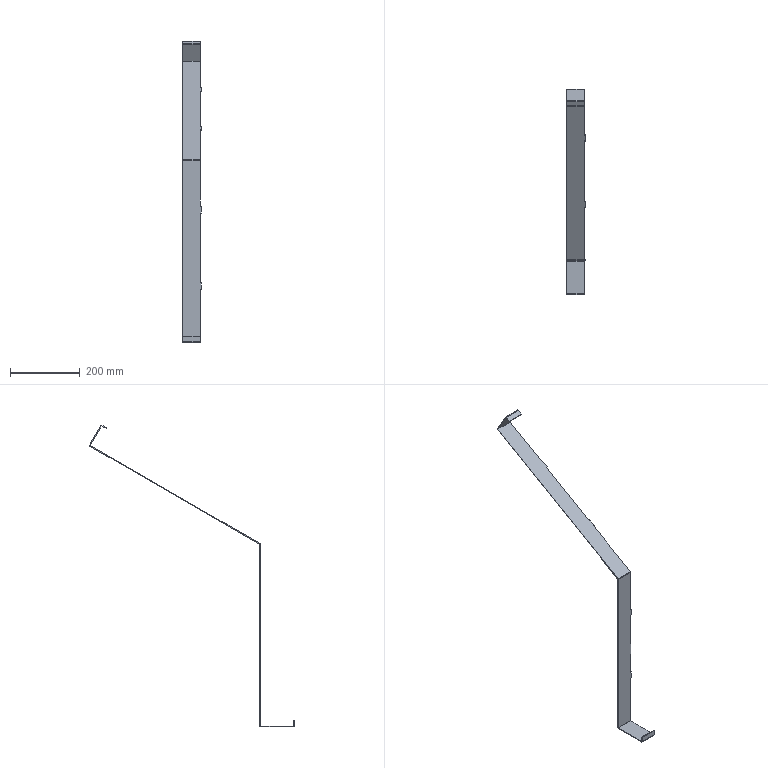Part | STEP file | zzh001 | 1 solid | 44 faces | box 53 x 587.725 x 864.748 mm | volume 128593 mm3 | plane 32 | cylinder 12 | commonest cylinder face diameters 1 x6 5 x6
STEP:
#1=CARTESIAN_POINT('',(50.,493.625,574.029));
#2=VERTEX_POINT('',#1);
#3=CARTESIAN_POINT('',(50.,494.058,573.779));
#4=VERTEX_POINT('',#3);
#5=CARTESIAN_POINT('',(50.,493.625,573.529));
#6=DIRECTION('',(-1.,0.,0.));
#7=DIRECTION('',(0.,0.,1.));
#8=AXIS2_PLACEMENT_3D('',#5,#6,#7);
#9=CIRCLE('',#8,0.5);
#10=EDGE_CURVE('',#2,#4,#9,.T.);
#11=ORIENTED_EDGE('',*,*,#10,.F.);
#12=CARTESIAN_POINT('',(0.,493.625,574.029));
#13=VERTEX_POINT('',#12);
#14=CARTESIAN_POINT('',(50.,493.625,574.029));
#15=DIRECTION('',(-1.,0.,0.));
#16=VECTOR('',#15,1000.);
#17=LINE('',#14,#16);
#18=EDGE_CURVE('',#2,#13,#17,.T.);
#19=ORIENTED_EDGE('',*,*,#18,.T.);
#20=CARTESIAN_POINT('',(0.,494.058,573.779));
#21=VERTEX_POINT('',#20);
#22=CARTESIAN_POINT('',(0.,493.625,573.529));
#23=DIRECTION('',(1.,0.,0.));
#24=DIRECTION('',(0.,0.,1.));
#25=AXIS2_PLACEMENT_3D('',#22,#23,#24);
#26=CIRCLE('',#25,0.5);
#27=EDGE_CURVE('',#21,#13,#26,.T.);
#28=ORIENTED_EDGE('',*,*,#27,.F.);
#29=CARTESIAN_POINT('',(50.,494.058,573.779));
#30=DIRECTION('',(-1.,0.,0.));
#31=VECTOR('',#30,1000.);
#32=LINE('',#29,#31);
#33=EDGE_CURVE('',#4,#21,#32,.T.);
#34=ORIENTED_EDGE('',*,*,#33,.F.);
#35=EDGE_LOOP('',(#11,#19,#28,#34));
#36=FACE_OUTER_BOUND('',#35,.T.);
#37=CARTESIAN_POINT('',(50.,493.625,573.529));
#38=DIRECTION('',(-1.,0.,0.));
#39=DIRECTION('',(0.,0.,1.));
#40=AXIS2_PLACEMENT_3D('',#37,#38,#39);
#41=CYLINDRICAL_SURFACE('',#40,0.5);
#42=ADVANCED_FACE('',(#36),#41,.F.);
#43=CARTESIAN_POINT('',(50.,493.625,576.029));
#44=VERTEX_POINT('',#43);
#45=CARTESIAN_POINT('',(50.,492.375,575.695));
#46=VERTEX_POINT('',#45);
#47=CARTESIAN_POINT('',(50.,493.625,573.529));
#48=DIRECTION('',(1.,0.,0.));
#49=DIRECTION('',(0.,0.,1.));
#50=AXIS2_PLACEMENT_3D('',#47,#48,#49);
#51=CIRCLE('',#50,2.5);
#52=EDGE_CURVE('',#44,#46,#51,.T.);
#53=ORIENTED_EDGE('',*,*,#52,.F.);
#54=CARTESIAN_POINT('',(0.,493.625,576.029));
#55=VERTEX_POINT('',#54);
#56=CARTESIAN_POINT('',(50.,493.625,576.029));
#57=DIRECTION('',(-1.,0.,0.));
#58=VECTOR('',#57,1000.);
#59=LINE('',#56,#58);
#60=EDGE_CURVE('',#44,#55,#59,.T.);
#61=ORIENTED_EDGE('',*,*,#60,.T.);
#62=CARTESIAN_POINT('',(0.,492.375,575.695));
#63=VERTEX_POINT('',#62);
#64=CARTESIAN_POINT('',(0.,493.625,573.529));
#65=DIRECTION('',(-1.,0.,0.));
#66=DIRECTION('',(0.,0.,1.));
#67=AXIS2_PLACEMENT_3D('',#64,#65,#66);
#68=CIRCLE('',#67,2.5);
#69=EDGE_CURVE('',#63,#55,#68,.T.);
#70=ORIENTED_EDGE('',*,*,#69,.F.);
#71=CARTESIAN_POINT('',(50.,492.375,575.695));
#72=DIRECTION('',(1.,0.,0.));
#73=VECTOR('',#72,1000.);
#74=LINE('',#71,#73);
#75=EDGE_CURVE('',#63,#46,#74,.T.);
#76=ORIENTED_EDGE('',*,*,#75,.T.);
#77=EDGE_LOOP('',(#53,#61,#70,#76));
#78=FACE_OUTER_BOUND('',#77,.T.);
#79=CARTESIAN_POINT('',(50.,493.625,573.529));
#80=DIRECTION('',(-1.,0.,0.));
#81=DIRECTION('',(0.,0.,1.));
#82=AXIS2_PLACEMENT_3D('',#79,#80,#81);
#83=CYLINDRICAL_SURFACE('',#82,2.5);
#84=ADVANCED_FACE('',(#78),#83,.T.);
#85=CARTESIAN_POINT('',(50.,396.504,442.748));
#86=VERTEX_POINT('',#85);
#87=CARTESIAN_POINT('',(50.,525.975,517.498));
#88=VERTEX_POINT('',#87);
#89=CARTESIAN_POINT('',(50.,37.7,235.592));
#90=DIRECTION('',(0.,0.866,0.5));
#91=VECTOR('',#90,1000.);
#92=LINE('',#89,#91);
#93=EDGE_CURVE('',#86,#88,#92,.T.);
#94=ORIENTED_EDGE('',*,*,#93,.T.);
#95=CARTESIAN_POINT('',(0.,525.975,517.498));
#96=VERTEX_POINT('',#95);
#97=CARTESIAN_POINT('',(50.,525.975,517.498));
#98=DIRECTION('',(-1.,0.,0.));
#99=VECTOR('',#98,1000.);
#100=LINE('',#97,#99);
#101=EDGE_CURVE('',#88,#96,#100,.T.);
#102=ORIENTED_EDGE('',*,*,#101,.T.);
#103=CARTESIAN_POINT('',(0.,38.95,236.314));
#104=VERTEX_POINT('',#103);
#105=CARTESIAN_POINT('',(0.,37.7,235.592));
#106=DIRECTION('',(0.,-0.866,-0.5));
#107=VECTOR('',#106,1000.);
#108=LINE('',#105,#107);
#109=EDGE_CURVE('',#96,#104,#108,.T.);
#110=ORIENTED_EDGE('',*,*,#109,.T.);
#111=CARTESIAN_POINT('',(50.,38.95,236.314));
#112=VERTEX_POINT('',#111);
#113=CARTESIAN_POINT('',(50.,38.95,236.314));
#114=DIRECTION('',(1.,0.,0.));
#115=VECTOR('',#114,1000.);
#116=LINE('',#113,#115);
#117=EDGE_CURVE('',#104,#112,#116,.T.);
#118=ORIENTED_EDGE('',*,*,#117,.T.);
#119=CARTESIAN_POINT('',(50.,188.658,322.748));
#120=VERTEX_POINT('',#119);
#121=CARTESIAN_POINT('',(50.,37.7,235.592));
#122=DIRECTION('',(0.,0.866,0.5));
#123=VECTOR('',#122,1000.);
#124=LINE('',#121,#123);
#125=EDGE_CURVE('',#112,#120,#124,.T.);
#126=ORIENTED_EDGE('',*,*,#125,.T.);
#127=CARTESIAN_POINT('',(53.,188.658,322.748));
#128=VERTEX_POINT('',#127);
#129=CARTESIAN_POINT('',(50.,188.658,322.748));
#130=DIRECTION('',(1.,0.,0.));
#131=VECTOR('',#130,1000.);
#132=LINE('',#129,#131);
#133=EDGE_CURVE('',#120,#128,#132,.T.);
#134=ORIENTED_EDGE('',*,*,#133,.T.);
#135=CARTESIAN_POINT('',(53.,205.978,332.748));
#136=VERTEX_POINT('',#135);
#137=CARTESIAN_POINT('',(53.,37.7,235.592));
#138=DIRECTION('',(0.,0.866,0.5));
#139=VECTOR('',#138,1000.);
#140=LINE('',#137,#139);
#141=EDGE_CURVE('',#128,#136,#140,.T.);
#142=ORIENTED_EDGE('',*,*,#141,.T.);
#143=CARTESIAN_POINT('',(50.,205.978,332.748));
#144=VERTEX_POINT('',#143);
#145=CARTESIAN_POINT('',(50.,205.978,332.748));
#146=DIRECTION('',(-1.,0.,0.));
#147=VECTOR('',#146,1000.);
#148=LINE('',#145,#147);
#149=EDGE_CURVE('',#136,#144,#148,.T.);
#150=ORIENTED_EDGE('',*,*,#149,.T.);
#151=CARTESIAN_POINT('',(50.,379.183,432.748));
#152=VERTEX_POINT('',#151);
#153=CARTESIAN_POINT('',(50.,37.7,235.592));
#154=DIRECTION('',(0.,0.866,0.5));
#155=VECTOR('',#154,1000.);
#156=LINE('',#153,#155);
#157=EDGE_CURVE('',#144,#152,#156,.T.);
#158=ORIENTED_EDGE('',*,*,#157,.T.);
#159=CARTESIAN_POINT('',(53.,379.183,432.748));
#160=VERTEX_POINT('',#159);
#161=CARTESIAN_POINT('',(50.,379.183,432.748));
#162=DIRECTION('',(1.,0.,0.));
#163=VECTOR('',#162,1000.);
#164=LINE('',#161,#163);
#165=EDGE_CURVE('',#152,#160,#164,.T.);
#166=ORIENTED_EDGE('',*,*,#165,.T.);
#167=CARTESIAN_POINT('',(53.,396.504,442.748));
#168=VERTEX_POINT('',#167);
#169=CARTESIAN_POINT('',(53.,37.7,235.592));
#170=DIRECTION('',(0.,0.866,0.5));
#171=VECTOR('',#170,1000.);
#172=LINE('',#169,#171);
#173=EDGE_CURVE('',#160,#168,#172,.T.);
#174=ORIENTED_EDGE('',*,*,#173,.T.);
#175=CARTESIAN_POINT('',(50.,396.504,442.748));
#176=DIRECTION('',(-1.,0.,0.));
#177=VECTOR('',#176,1000.);
#178=LINE('',#175,#177);
#179=EDGE_CURVE('',#168,#86,#178,.T.);
#180=ORIENTED_EDGE('',*,*,#179,.T.);
#181=EDGE_LOOP('',(#94,#102,#110,#118,#126,#134,#142,#150,#158,#166,#174,#180));
#182=FACE_OUTER_BOUND('',#181,.T.);
#183=CARTESIAN_POINT('',(50.,37.7,235.592));
#184=DIRECTION('',(0.,-0.5,0.866));
#185=DIRECTION('',(0.,-0.866,-0.5));
#186=AXIS2_PLACEMENT_3D('',#183,#184,#185);
#187=PLANE('',#186);
#188=ADVANCED_FACE('',(#182),#187,.T.);
#189=ORIENTED_EDGE('',*,*,#101,.F.);
#190=CARTESIAN_POINT('',(50.,526.158,518.181));
#191=VERTEX_POINT('',#190);
#192=CARTESIAN_POINT('',(50.,525.725,517.931));
#193=DIRECTION('',(-1.,0.,0.));
#194=DIRECTION('',(0.,0.,1.));
#195=AXIS2_PLACEMENT_3D('',#192,#193,#194);
#196=CIRCLE('',#195,0.5);
#197=EDGE_CURVE('',#191,#88,#196,.T.);
#198=ORIENTED_EDGE('',*,*,#197,.F.);
#199=CARTESIAN_POINT('',(0.,526.158,518.181));
#200=VERTEX_POINT('',#199);
#201=CARTESIAN_POINT('',(50.,526.158,518.181));
#202=DIRECTION('',(1.,0.,0.));
#203=VECTOR('',#202,1000.);
#204=LINE('',#201,#203);
#205=EDGE_CURVE('',#200,#191,#204,.T.);
#206=ORIENTED_EDGE('',*,*,#205,.F.);
#207=CARTESIAN_POINT('',(0.,525.725,517.931));
#208=DIRECTION('',(1.,0.,0.));
#209=DIRECTION('',(0.,0.,1.));
#210=AXIS2_PLACEMENT_3D('',#207,#208,#209);
#211=CIRCLE('',#210,0.5);
#212=EDGE_CURVE('',#96,#200,#211,.T.);
#213=ORIENTED_EDGE('',*,*,#212,.F.);
#214=EDGE_LOOP('',(#189,#198,#206,#213));
#215=FACE_OUTER_BOUND('',#214,.T.);
#216=CARTESIAN_POINT('',(50.,525.725,517.931));
#217=DIRECTION('',(-1.,0.,0.));
#218=DIRECTION('',(0.,0.,1.));
#219=AXIS2_PLACEMENT_3D('',#216,#217,#218);
#220=CYLINDRICAL_SURFACE('',#219,0.5);
#221=ADVANCED_FACE('',(#215),#220,.F.);
#222=CARTESIAN_POINT('',(50.,397.504,441.016));
#223=VERTEX_POINT('',#222);
#224=CARTESIAN_POINT('',(50.,526.975,515.766));
#225=VERTEX_POINT('',#224);
#226=CARTESIAN_POINT('',(50.,397.504,441.016));
#227=DIRECTION('',(0.,0.866,0.5));
#228=VECTOR('',#227,1000.);
#229=LINE('',#226,#228);
#230=EDGE_CURVE('',#223,#225,#229,.T.);
#231=ORIENTED_EDGE('',*,*,#230,.T.);
#232=CARTESIAN_POINT('',(50.,527.89,519.181));
#233=VERTEX_POINT('',#232);
#234=CARTESIAN_POINT('',(50.,525.725,517.931));
#235=DIRECTION('',(1.,0.,0.));
#236=DIRECTION('',(0.,0.,1.));
#237=AXIS2_PLACEMENT_3D('',#234,#235,#236);
#238=CIRCLE('',#237,2.5);
#239=EDGE_CURVE('',#225,#233,#238,.T.);
#240=ORIENTED_EDGE('',*,*,#239,.T.);
#241=CARTESIAN_POINT('',(50.,495.79,574.779));
#242=VERTEX_POINT('',#241);
#243=CARTESIAN_POINT('',(50.,527.89,519.181));
#244=DIRECTION('',(0.,-0.5,0.866));
#245=VECTOR('',#244,1000.);
#246=LINE('',#243,#245);
#247=EDGE_CURVE('',#233,#242,#246,.T.);
#248=ORIENTED_EDGE('',*,*,#247,.T.);
#249=CARTESIAN_POINT('',(50.,493.625,573.529));
#250=DIRECTION('',(1.,0.,0.));
#251=DIRECTION('',(0.,0.,1.));
#252=AXIS2_PLACEMENT_3D('',#249,#250,#251);
#253=CIRCLE('',#252,2.5);
#254=EDGE_CURVE('',#242,#44,#253,.T.);
#255=ORIENTED_EDGE('',*,*,#254,.T.);
#256=ORIENTED_EDGE('',*,*,#52,.T.);
#257=CARTESIAN_POINT('',(50.,479.817,568.445));
#258=VERTEX_POINT('',#257);
#259=CARTESIAN_POINT('',(50.,492.375,575.695));
#260=DIRECTION('',(0.,-0.866,-0.5));
#261=VECTOR('',#260,1000.);
#262=LINE('',#259,#261);
#263=EDGE_CURVE('',#46,#258,#262,.T.);
#264=ORIENTED_EDGE('',*,*,#263,.T.);
#265=CARTESIAN_POINT('',(50.,480.817,566.713));
#266=VERTEX_POINT('',#265);
#267=CARTESIAN_POINT('',(50.,479.817,568.445));
#268=DIRECTION('',(0.,0.5,-0.866));
#269=VECTOR('',#268,1000.);
#270=LINE('',#267,#269);
#271=EDGE_CURVE('',#258,#266,#270,.T.);
#272=ORIENTED_EDGE('',*,*,#271,.T.);
#273=CARTESIAN_POINT('',(50.,493.375,573.963));
#274=VERTEX_POINT('',#273);
#275=CARTESIAN_POINT('',(50.,493.808,574.213));
#276=DIRECTION('',(0.,-0.866,-0.5));
#277=VECTOR('',#276,1000.);
#278=LINE('',#275,#277);
#279=EDGE_CURVE('',#274,#266,#278,.T.);
#280=ORIENTED_EDGE('',*,*,#279,.F.);
#281=CARTESIAN_POINT('',(50.,493.625,573.529));
#282=DIRECTION('',(-1.,0.,0.));
#283=DIRECTION('',(0.,0.,1.));
#284=AXIS2_PLACEMENT_3D('',#281,#282,#283);
#285=CIRCLE('',#284,0.5);
#286=EDGE_CURVE('',#274,#2,#285,.T.);
#287=ORIENTED_EDGE('',*,*,#286,.T.);
#288=ORIENTED_EDGE('',*,*,#10,.T.);
#289=CARTESIAN_POINT('',(50.,526.408,517.748));
#290=DIRECTION('',(0.,-0.5,0.866));
#291=VECTOR('',#290,1000.);
#292=LINE('',#289,#291);
#293=EDGE_CURVE('',#191,#4,#292,.T.);
#294=ORIENTED_EDGE('',*,*,#293,.F.);
#295=ORIENTED_EDGE('',*,*,#197,.T.);
#296=ORIENTED_EDGE('',*,*,#93,.F.);
#297=CARTESIAN_POINT('',(50.,396.504,442.748));
#298=DIRECTION('',(0.,0.5,-0.866));
#299=VECTOR('',#298,1000.);
#300=LINE('',#297,#299);
#301=EDGE_CURVE('',#86,#223,#300,.T.);
#302=ORIENTED_EDGE('',*,*,#301,.T.);
#303=EDGE_LOOP('',(#231,#240,#248,#255,#256,#264,#272,#280,#287,#288,#294,#295,#296,#302));
#304=FACE_OUTER_BOUND('',#303,.T.);
#305=CARTESIAN_POINT('',(50.,39.7,234.149));
#306=DIRECTION('',(1.,0.,0.));
#307=DIRECTION('',(0.,0.,-1.));
#308=AXIS2_PLACEMENT_3D('',#305,#306,#307);
#309=PLANE('',#308);
#310=ADVANCED_FACE('',(#304),#309,.T.);
#311=ORIENTED_EDGE('',*,*,#179,.F.);
#312=CARTESIAN_POINT('',(53.,397.504,441.016));
#313=VERTEX_POINT('',#312);
#314=CARTESIAN_POINT('',(53.,396.504,442.748));
#315=DIRECTION('',(0.,-0.5,0.866));
#316=VECTOR('',#315,1000.);
#317=LINE('',#314,#316);
#318=EDGE_CURVE('',#313,#168,#317,.T.);
#319=ORIENTED_EDGE('',*,*,#318,.F.);
#320=CARTESIAN_POINT('',(53.,397.504,441.016));
#321=DIRECTION('',(1.,0.,0.));
#322=VECTOR('',#321,1000.);
#323=LINE('',#320,#322);
#324=EDGE_CURVE('',#223,#313,#323,.T.);
#325=ORIENTED_EDGE('',*,*,#324,.F.);
#326=ORIENTED_EDGE('',*,*,#301,.F.);
#327=EDGE_LOOP('',(#311,#319,#325,#326));
#328=FACE_OUTER_BOUND('',#327,.T.);
#329=CARTESIAN_POINT('',(53.,396.504,442.748));
#330=DIRECTION('',(0.,-0.866,-0.5));
#331=DIRECTION('',(0.,0.5,-0.866));
#332=AXIS2_PLACEMENT_3D('',#329,#330,#331);
#333=PLANE('',#332);
#334=ADVANCED_FACE('',(#328),#333,.F.);
#335=ORIENTED_EDGE('',*,*,#173,.F.);
#336=CARTESIAN_POINT('',(53.,380.183,431.016));
#337=VERTEX_POINT('',#336);
#338=CARTESIAN_POINT('',(53.,380.183,431.016));
#339=DIRECTION('',(0.,-0.5,0.866));
#340=VECTOR('',#339,1000.);
#341=LINE('',#338,#340);
#342=EDGE_CURVE('',#337,#160,#341,.T.);
#343=ORIENTED_EDGE('',*,*,#342,.F.);
#344=CARTESIAN_POINT('',(53.,397.504,441.016));
#345=DIRECTION('',(0.,-0.866,-0.5));
#346=VECTOR('',#345,1000.);
#347=LINE('',#344,#346);
#348=EDGE_CURVE('',#313,#337,#347,.T.);
#349=ORIENTED_EDGE('',*,*,#348,.F.);
#350=ORIENTED_EDGE('',*,*,#318,.T.);
#351=EDGE_LOOP('',(#335,#343,#349,#350));
#352=FACE_OUTER_BOUND('',#351,.T.);
#353=CARTESIAN_POINT('',(53.,0.,0.));
#354=DIRECTION('',(-1.,0.,0.));
#355=DIRECTION('',(0.,0.,1.));
#356=AXIS2_PLACEMENT_3D('',#353,#354,#355);
#357=PLANE('',#356);
#358=ADVANCED_FACE('',(#352),#357,.F.);
#359=CARTESIAN_POINT('',(50.,380.183,431.016));
#360=VERTEX_POINT('',#359);
#361=CARTESIAN_POINT('',(53.,380.183,431.016));
#362=DIRECTION('',(-1.,0.,0.));
#363=VECTOR('',#362,1000.);
#364=LINE('',#361,#363);
#365=EDGE_CURVE('',#337,#360,#364,.T.);
#366=ORIENTED_EDGE('',*,*,#365,.F.);
#367=ORIENTED_EDGE('',*,*,#342,.T.);
#368=ORIENTED_EDGE('',*,*,#165,.F.);
#369=CARTESIAN_POINT('',(50.,379.183,432.748));
#370=DIRECTION('',(0.,-0.5,0.866));
#371=VECTOR('',#370,1000.);
#372=LINE('',#369,#371);
#373=EDGE_CURVE('',#360,#152,#372,.T.);
#374=ORIENTED_EDGE('',*,*,#373,.F.);
#375=EDGE_LOOP('',(#366,#367,#368,#374));
#376=FACE_OUTER_BOUND('',#375,.T.);
#377=CARTESIAN_POINT('',(53.,379.183,432.748));
#378=DIRECTION('',(0.,0.866,0.5));
#379=DIRECTION('',(0.,-0.5,0.866));
#380=AXIS2_PLACEMENT_3D('',#377,#378,#379);
#381=PLANE('',#380);
#382=ADVANCED_FACE('',(#376),#381,.F.);
#383=CARTESIAN_POINT('',(50.,206.978,331.016));
#384=VERTEX_POINT('',#383);
#385=CARTESIAN_POINT('',(50.,206.978,331.016));
#386=DIRECTION('',(0.,0.866,0.5));
#387=VECTOR('',#386,1000.);
#388=LINE('',#385,#387);
#389=EDGE_CURVE('',#384,#360,#388,.T.);
#390=ORIENTED_EDGE('',*,*,#389,.T.);
#391=ORIENTED_EDGE('',*,*,#373,.T.);
#392=ORIENTED_EDGE('',*,*,#157,.F.);
#393=CARTESIAN_POINT('',(50.,205.978,332.748));
#394=DIRECTION('',(0.,0.5,-0.866));
#395=VECTOR('',#394,1000.);
#396=LINE('',#393,#395);
#397=EDGE_CURVE('',#144,#384,#396,.T.);
#398=ORIENTED_EDGE('',*,*,#397,.T.);
#399=EDGE_LOOP('',(#390,#391,#392,#398));
#400=FACE_OUTER_BOUND('',#399,.T.);
#401=CARTESIAN_POINT('',(50.,39.7,234.149));
#402=DIRECTION('',(1.,0.,0.));
#403=DIRECTION('',(0.,0.,-1.));
#404=AXIS2_PLACEMENT_3D('',#401,#402,#403);
#405=PLANE('',#404);
#406=ADVANCED_FACE('',(#400),#405,.T.);
#407=ORIENTED_EDGE('',*,*,#149,.F.);
#408=CARTESIAN_POINT('',(53.,206.978,331.016));
#409=VERTEX_POINT('',#408);
#410=CARTESIAN_POINT('',(53.,205.978,332.748));
#411=DIRECTION('',(0.,-0.5,0.866));
#412=VECTOR('',#411,1000.);
#413=LINE('',#410,#412);
#414=EDGE_CURVE('',#409,#136,#413,.T.);
#415=ORIENTED_EDGE('',*,*,#414,.F.);
#416=CARTESIAN_POINT('',(53.,206.978,331.016));
#417=DIRECTION('',(1.,0.,0.));
#418=VECTOR('',#417,1000.);
#419=LINE('',#416,#418);
#420=EDGE_CURVE('',#384,#409,#419,.T.);
#421=ORIENTED_EDGE('',*,*,#420,.F.);
#422=ORIENTED_EDGE('',*,*,#397,.F.);
#423=EDGE_LOOP('',(#407,#415,#421,#422));
#424=FACE_OUTER_BOUND('',#423,.T.);
#425=CARTESIAN_POINT('',(53.,205.978,332.748));
#426=DIRECTION('',(0.,-0.866,-0.5));
#427=DIRECTION('',(0.,0.5,-0.866));
#428=AXIS2_PLACEMENT_3D('',#425,#426,#427);
#429=PLANE('',#428);
#430=ADVANCED_FACE('',(#424),#429,.F.);
#431=ORIENTED_EDGE('',*,*,#141,.F.);
#432=CARTESIAN_POINT('',(53.,189.658,321.016));
#433=VERTEX_POINT('',#432);
#434=CARTESIAN_POINT('',(53.,189.658,321.016));
#435=DIRECTION('',(0.,-0.5,0.866));
#436=VECTOR('',#435,1000.);
#437=LINE('',#434,#436);
#438=EDGE_CURVE('',#433,#128,#437,.T.);
#439=ORIENTED_EDGE('',*,*,#438,.F.);
#440=CARTESIAN_POINT('',(53.,206.978,331.016));
#441=DIRECTION('',(0.,-0.866,-0.5));
#442=VECTOR('',#441,1000.);
#443=LINE('',#440,#442);
#444=EDGE_CURVE('',#409,#433,#443,.T.);
#445=ORIENTED_EDGE('',*,*,#444,.F.);
#446=ORIENTED_EDGE('',*,*,#414,.T.);
#447=EDGE_LOOP('',(#431,#439,#445,#446));
#448=FACE_OUTER_BOUND('',#447,.T.);
#449=CARTESIAN_POINT('',(53.,0.,0.));
#450=DIRECTION('',(-1.,0.,0.));
#451=DIRECTION('',(0.,0.,1.));
#452=AXIS2_PLACEMENT_3D('',#449,#450,#451);
#453=PLANE('',#452);
#454=ADVANCED_FACE('',(#448),#453,.F.);
#455=CARTESIAN_POINT('',(50.,189.658,321.016));
#456=VERTEX_POINT('',#455);
#457=CARTESIAN_POINT('',(53.,189.658,321.016));
#458=DIRECTION('',(-1.,0.,0.));
#459=VECTOR('',#458,1000.);
#460=LINE('',#457,#459);
#461=EDGE_CURVE('',#433,#456,#460,.T.);
#462=ORIENTED_EDGE('',*,*,#461,.F.);
#463=ORIENTED_EDGE('',*,*,#438,.T.);
#464=ORIENTED_EDGE('',*,*,#133,.F.);
#465=CARTESIAN_POINT('',(50.,188.658,322.748));
#466=DIRECTION('',(0.,-0.5,0.866));
#467=VECTOR('',#466,1000.);
#468=LINE('',#465,#467);
#469=EDGE_CURVE('',#456,#120,#468,.T.);
#470=ORIENTED_EDGE('',*,*,#469,.F.);
#471=EDGE_LOOP('',(#462,#463,#464,#470));
#472=FACE_OUTER_BOUND('',#471,.T.);
#473=CARTESIAN_POINT('',(53.,188.658,322.748));
#474=DIRECTION('',(0.,0.866,0.5));
#475=DIRECTION('',(0.,-0.5,0.866));
#476=AXIS2_PLACEMENT_3D('',#473,#474,#475);
#477=PLANE('',#476);
#478=ADVANCED_FACE('',(#472),#477,.F.);
#479=ORIENTED_EDGE('',*,*,#125,.F.);
#480=CARTESIAN_POINT('',(50.,37.7,234.149));
#481=VERTEX_POINT('',#480);
#482=CARTESIAN_POINT('',(50.,40.2,234.149));
#483=DIRECTION('',(-1.,0.,0.));
#484=DIRECTION('',(0.,0.,1.));
#485=AXIS2_PLACEMENT_3D('',#482,#483,#484);
#486=CIRCLE('',#485,2.5);
#487=EDGE_CURVE('',#481,#112,#486,.T.);
#488=ORIENTED_EDGE('',*,*,#487,.F.);
#489=CARTESIAN_POINT('',(50.,37.7,103.281));
#490=VERTEX_POINT('',#489);
#491=CARTESIAN_POINT('',(50.,37.7,-286.719));
#492=DIRECTION('',(0.,0.,1.));
#493=VECTOR('',#492,1000.);
#494=LINE('',#491,#493);
#495=EDGE_CURVE('',#490,#481,#494,.T.);
#496=ORIENTED_EDGE('',*,*,#495,.F.);
#497=CARTESIAN_POINT('',(50.,39.7,103.281));
#498=VERTEX_POINT('',#497);
#499=CARTESIAN_POINT('',(50.,37.2,103.281));
#500=DIRECTION('',(0.,1.,0.));
#501=VECTOR('',#500,1000.);
#502=LINE('',#499,#501);
#503=EDGE_CURVE('',#490,#498,#502,.T.);
#504=ORIENTED_EDGE('',*,*,#503,.T.);
#505=CARTESIAN_POINT('',(50.,39.7,234.149));
#506=VERTEX_POINT('',#505);
#507=CARTESIAN_POINT('',(50.,39.7,-288.719));
#508=DIRECTION('',(0.,0.,1.));
#509=VECTOR('',#508,1000.);
#510=LINE('',#507,#509);
#511=EDGE_CURVE('',#498,#506,#510,.T.);
#512=ORIENTED_EDGE('',*,*,#511,.T.);
#513=CARTESIAN_POINT('',(50.,39.95,234.582));
#514=VERTEX_POINT('',#513);
#515=CARTESIAN_POINT('',(50.,40.2,234.149));
#516=DIRECTION('',(-1.,0.,0.));
#517=DIRECTION('',(0.,0.,1.));
#518=AXIS2_PLACEMENT_3D('',#515,#516,#517);
#519=CIRCLE('',#518,0.5);
#520=EDGE_CURVE('',#506,#514,#519,.T.);
#521=ORIENTED_EDGE('',*,*,#520,.T.);
#522=CARTESIAN_POINT('',(50.,39.95,234.582));
#523=DIRECTION('',(0.,0.866,0.5));
#524=VECTOR('',#523,1000.);
#525=LINE('',#522,#524);
#526=EDGE_CURVE('',#514,#456,#525,.T.);
#527=ORIENTED_EDGE('',*,*,#526,.T.);
#528=ORIENTED_EDGE('',*,*,#469,.T.);
#529=EDGE_LOOP('',(#479,#488,#496,#504,#512,#521,#527,#528));
#530=FACE_OUTER_BOUND('',#529,.T.);
#531=CARTESIAN_POINT('',(50.,39.7,234.149));
#532=DIRECTION('',(1.,0.,0.));
#533=DIRECTION('',(0.,0.,-1.));
#534=AXIS2_PLACEMENT_3D('',#531,#532,#533);
#535=PLANE('',#534);
#536=ADVANCED_FACE('',(#530),#535,.T.);
#537=ORIENTED_EDGE('',*,*,#487,.T.);
#538=ORIENTED_EDGE('',*,*,#117,.F.);
#539=CARTESIAN_POINT('',(0.,37.7,234.149));
#540=VERTEX_POINT('',#539);
#541=CARTESIAN_POINT('',(0.,40.2,234.149));
#542=DIRECTION('',(1.,0.,0.));
#543=DIRECTION('',(0.,0.,1.));
#544=AXIS2_PLACEMENT_3D('',#541,#542,#543);
#545=CIRCLE('',#544,2.5);
#546=EDGE_CURVE('',#104,#540,#545,.T.);
#547=ORIENTED_EDGE('',*,*,#546,.T.);
#548=CARTESIAN_POINT('',(50.,37.7,234.149));
#549=DIRECTION('',(1.,0.,0.));
#550=VECTOR('',#549,1000.);
#551=LINE('',#548,#550);
#552=EDGE_CURVE('',#540,#481,#551,.T.);
#553=ORIENTED_EDGE('',*,*,#552,.T.);
#554=EDGE_LOOP('',(#537,#538,#547,#553));
#555=FACE_OUTER_BOUND('',#554,.T.);
#556=CARTESIAN_POINT('',(50.,40.2,234.149));
#557=DIRECTION('',(-1.,0.,0.));
#558=DIRECTION('',(0.,0.,1.));
#559=AXIS2_PLACEMENT_3D('',#556,#557,#558);
#560=CYLINDRICAL_SURFACE('',#559,2.5);
#561=ADVANCED_FACE('',(#555),#560,.T.);
#562=CARTESIAN_POINT('',(0.,526.975,515.766));
#563=VERTEX_POINT('',#562);
#564=CARTESIAN_POINT('',(0.,39.95,234.582));
#565=VERTEX_POINT('',#564);
#566=CARTESIAN_POINT('',(0.,526.975,515.766));
#567=DIRECTION('',(0.,-0.866,-0.5));
#568=VECTOR('',#567,1000.);
#569=LINE('',#566,#568);
#570=EDGE_CURVE('',#563,#565,#569,.T.);
#571=ORIENTED_EDGE('',*,*,#570,.T.);
#572=CARTESIAN_POINT('',(0.,39.7,234.149));
#573=VERTEX_POINT('',#572);
#574=CARTESIAN_POINT('',(0.,40.2,234.149));
#575=DIRECTION('',(1.,0.,0.));
#576=DIRECTION('',(0.,0.,1.));
#577=AXIS2_PLACEMENT_3D('',#574,#575,#576);
#578=CIRCLE('',#577,0.5);
#579=EDGE_CURVE('',#565,#573,#578,.T.);
#580=ORIENTED_EDGE('',*,*,#579,.T.);
#581=CARTESIAN_POINT('',(0.,39.7,-286.219));
#582=VERTEX_POINT('',#581);
#583=CARTESIAN_POINT('',(0.,39.7,234.582));
#584=DIRECTION('',(0.,0.,-1.));
#585=VECTOR('',#584,1000.);
#586=LINE('',#583,#585);
#587=EDGE_CURVE('',#573,#582,#586,.T.);
#588=ORIENTED_EDGE('',*,*,#587,.T.);
#589=CARTESIAN_POINT('',(0.,37.2,-288.719));
#590=VERTEX_POINT('',#589);
#591=CARTESIAN_POINT('',(0.,37.2,-286.219));
#592=DIRECTION('',(-1.,0.,0.));
#593=DIRECTION('',(0.,0.,1.));
#594=AXIS2_PLACEMENT_3D('',#591,#592,#593);
#595=CIRCLE('',#594,2.5);
#596=EDGE_CURVE('',#582,#590,#595,.T.);
#597=ORIENTED_EDGE('',*,*,#596,.T.);
#598=CARTESIAN_POINT('',(0.,-57.,-288.719));
#599=VERTEX_POINT('',#598);
#600=CARTESIAN_POINT('',(0.,39.7,-288.719));
#601=DIRECTION('',(0.,-1.,0.));
#602=VECTOR('',#601,1000.);
#603=LINE('',#600,#602);
#604=EDGE_CURVE('',#590,#599,#603,.T.);
#605=ORIENTED_EDGE('',*,*,#604,.T.);
#606=CARTESIAN_POINT('',(0.,-59.5,-286.219));
#607=VERTEX_POINT('',#606);
#608=CARTESIAN_POINT('',(0.,-57.,-286.219));
#609=DIRECTION('',(-1.,0.,0.));
#610=DIRECTION('',(0.,0.,1.));
#611=AXIS2_PLACEMENT_3D('',#608,#609,#610);
#612=CIRCLE('',#611,2.5);
#613=EDGE_CURVE('',#599,#607,#612,.T.);
#614=ORIENTED_EDGE('',*,*,#613,.T.);
#615=CARTESIAN_POINT('',(0.,-59.5,-271.719));
#616=VERTEX_POINT('',#615);
#617=CARTESIAN_POINT('',(0.,-59.5,-288.719));
#618=DIRECTION('',(0.,0.,1.));
#619=VECTOR('',#618,1000.);
#620=LINE('',#617,#619);
#621=EDGE_CURVE('',#607,#616,#620,.T.);
#622=ORIENTED_EDGE('',*,*,#621,.T.);
#623=CARTESIAN_POINT('',(0.,-57.5,-271.719));
#624=VERTEX_POINT('',#623);
#625=CARTESIAN_POINT('',(0.,-59.5,-271.719));
#626=DIRECTION('',(0.,-1.,0.));
#627=VECTOR('',#626,1000.);
#628=LINE('',#625,#627);
#629=EDGE_CURVE('',#624,#616,#628,.T.);
#630=ORIENTED_EDGE('',*,*,#629,.F.);
#631=CARTESIAN_POINT('',(0.,-57.5,-286.219));
#632=VERTEX_POINT('',#631);
#633=CARTESIAN_POINT('',(0.,-57.5,-286.719));
#634=DIRECTION('',(0.,0.,1.));
#635=VECTOR('',#634,1000.);
#636=LINE('',#633,#635);
#637=EDGE_CURVE('',#632,#624,#636,.T.);
#638=ORIENTED_EDGE('',*,*,#637,.F.);
#639=CARTESIAN_POINT('',(0.,-57.,-286.719));
#640=VERTEX_POINT('',#639);
#641=CARTESIAN_POINT('',(0.,-57.,-286.219));
#642=DIRECTION('',(1.,0.,0.));
#643=DIRECTION('',(0.,0.,1.));
#644=AXIS2_PLACEMENT_3D('',#641,#642,#643);
#645=CIRCLE('',#644,0.5);
#646=EDGE_CURVE('',#632,#640,#645,.T.);
#647=ORIENTED_EDGE('',*,*,#646,.T.);
#648=CARTESIAN_POINT('',(0.,37.2,-286.719));
#649=VERTEX_POINT('',#648);
#650=CARTESIAN_POINT('',(0.,-52.5,-286.719));
#651=DIRECTION('',(0.,-1.,0.));
#652=VECTOR('',#651,1000.);
#653=LINE('',#650,#652);
#654=EDGE_CURVE('',#649,#640,#653,.T.);
#655=ORIENTED_EDGE('',*,*,#654,.F.);
#656=CARTESIAN_POINT('',(0.,37.7,-286.219));
#657=VERTEX_POINT('',#656);
#658=CARTESIAN_POINT('',(0.,37.2,-286.219));
#659=DIRECTION('',(1.,0.,0.));
#660=DIRECTION('',(0.,0.,1.));
#661=AXIS2_PLACEMENT_3D('',#658,#659,#660);
#662=CIRCLE('',#661,0.5);
#663=EDGE_CURVE('',#649,#657,#662,.T.);
#664=ORIENTED_EDGE('',*,*,#663,.T.);
#665=CARTESIAN_POINT('',(0.,37.7,-286.719));
#666=DIRECTION('',(0.,0.,-1.));
#667=VECTOR('',#666,1000.);
#668=LINE('',#665,#667);
#669=EDGE_CURVE('',#540,#657,#668,.T.);
#670=ORIENTED_EDGE('',*,*,#669,.F.);
#671=ORIENTED_EDGE('',*,*,#546,.F.);
#672=ORIENTED_EDGE('',*,*,#109,.F.);
#673=ORIENTED_EDGE('',*,*,#212,.T.);
#674=CARTESIAN_POINT('',(0.,526.408,517.748));
#675=DIRECTION('',(0.,0.5,-0.866));
#676=VECTOR('',#675,1000.);
#677=LINE('',#674,#676);
#678=EDGE_CURVE('',#21,#200,#677,.T.);
#679=ORIENTED_EDGE('',*,*,#678,.F.);
#680=ORIENTED_EDGE('',*,*,#27,.T.);
#681=CARTESIAN_POINT('',(0.,493.375,573.963));
#682=VERTEX_POINT('',#681);
#683=CARTESIAN_POINT('',(0.,493.625,573.529));
#684=DIRECTION('',(1.,0.,0.));
#685=DIRECTION('',(0.,0.,1.));
#686=AXIS2_PLACEMENT_3D('',#683,#684,#685);
#687=CIRCLE('',#686,0.5);
#688=EDGE_CURVE('',#13,#682,#687,.T.);
#689=ORIENTED_EDGE('',*,*,#688,.T.);
#690=CARTESIAN_POINT('',(0.,480.817,566.713));
#691=VERTEX_POINT('',#690);
#692=CARTESIAN_POINT('',(0.,493.808,574.213));
#693=DIRECTION('',(0.,0.866,0.5));
#694=VECTOR('',#693,1000.);
#695=LINE('',#692,#694);
#696=EDGE_CURVE('',#691,#682,#695,.T.);
#697=ORIENTED_EDGE('',*,*,#696,.F.);
#698=CARTESIAN_POINT('',(0.,479.817,568.445));
#699=VERTEX_POINT('',#698);
#700=CARTESIAN_POINT('',(0.,480.817,566.713));
#701=DIRECTION('',(0.,-0.5,0.866));
#702=VECTOR('',#701,1000.);
#703=LINE('',#700,#702);
#704=EDGE_CURVE('',#691,#699,#703,.T.);
#705=ORIENTED_EDGE('',*,*,#704,.T.);
#706=CARTESIAN_POINT('',(0.,479.817,568.445));
#707=DIRECTION('',(0.,0.866,0.5));
#708=VECTOR('',#707,1000.);
#709=LINE('',#706,#708);
#710=EDGE_CURVE('',#699,#63,#709,.T.);
#711=ORIENTED_EDGE('',*,*,#710,.T.);
#712=ORIENTED_EDGE('',*,*,#69,.T.);
#713=CARTESIAN_POINT('',(0.,495.79,574.779));
#714=VERTEX_POINT('',#713);
#715=CARTESIAN_POINT('',(0.,493.625,573.529));
#716=DIRECTION('',(-1.,0.,0.));
#717=DIRECTION('',(0.,0.,1.));
#718=AXIS2_PLACEMENT_3D('',#715,#716,#717);
#719=CIRCLE('',#718,2.5);
#720=EDGE_CURVE('',#55,#714,#719,.T.);
#721=ORIENTED_EDGE('',*,*,#720,.T.);
#722=CARTESIAN_POINT('',(0.,527.89,519.181));
#723=VERTEX_POINT('',#722);
#724=CARTESIAN_POINT('',(0.,495.79,574.779));
#725=DIRECTION('',(0.,0.5,-0.866));
#726=VECTOR('',#725,1000.);
#727=LINE('',#724,#726);
#728=EDGE_CURVE('',#714,#723,#727,.T.);
#729=ORIENTED_EDGE('',*,*,#728,.T.);
#730=CARTESIAN_POINT('',(0.,525.725,517.931));
#731=DIRECTION('',(-1.,0.,0.));
#732=DIRECTION('',(0.,0.,1.));
#733=AXIS2_PLACEMENT_3D('',#730,#731,#732);
#734=CIRCLE('',#733,2.5);
#735=EDGE_CURVE('',#723,#563,#734,.T.);
#736=ORIENTED_EDGE('',*,*,#735,.T.);
#737=EDGE_LOOP('',(#571,#580,#588,#597,#605,#614,#622,#630,#638,#647,#655,#664,#670,#671,#672,#673,#679,#680,#689,#697,#705,#711,#712,#721,#729,#736));
#738=FACE_OUTER_BOUND('',#737,.T.);
#739=CARTESIAN_POINT('',(0.,527.89,519.181));
#740=DIRECTION('',(-1.,0.,0.));
#741=DIRECTION('',(0.,0.,1.));
#742=AXIS2_PLACEMENT_3D('',#739,#740,#741);
#743=PLANE('',#742);
#744=ADVANCED_FACE('',(#738),#743,.T.);
#745=ORIENTED_EDGE('',*,*,#293,.T.);
#746=ORIENTED_EDGE('',*,*,#33,.T.);
#747=ORIENTED_EDGE('',*,*,#678,.T.);
#748=ORIENTED_EDGE('',*,*,#205,.T.);
#749=EDGE_LOOP('',(#745,#746,#747,#748));
#750=FACE_OUTER_BOUND('',#749,.T.);
#751=CARTESIAN_POINT('',(50.,526.408,517.748));
#752=DIRECTION('',(0.,-0.866,-0.5));
#753=DIRECTION('',(0.,0.5,-0.866));
#754=AXIS2_PLACEMENT_3D('',#751,#752,#753);
#755=PLANE('',#754);
#756=ADVANCED_FACE('',(#750),#755,.T.);
#757=CARTESIAN_POINT('',(50.,526.975,515.766));
#758=DIRECTION('',(-1.,0.,0.));
#759=VECTOR('',#758,1000.);
#760=LINE('',#757,#759);
#761=EDGE_CURVE('',#225,#563,#760,.T.);
#762=ORIENTED_EDGE('',*,*,#761,.F.);
#763=ORIENTED_EDGE('',*,*,#230,.F.);
#764=ORIENTED_EDGE('',*,*,#324,.T.);
#765=ORIENTED_EDGE('',*,*,#348,.T.);
#766=ORIENTED_EDGE('',*,*,#365,.T.);
#767=ORIENTED_EDGE('',*,*,#389,.F.);
#768=ORIENTED_EDGE('',*,*,#420,.T.);
#769=ORIENTED_EDGE('',*,*,#444,.T.);
#770=ORIENTED_EDGE('',*,*,#461,.T.);
#771=ORIENTED_EDGE('',*,*,#526,.F.);
#772=CARTESIAN_POINT('',(50.,39.95,234.582));
#773=DIRECTION('',(1.,0.,0.));
#774=VECTOR('',#773,1000.);
#775=LINE('',#772,#774);
#776=EDGE_CURVE('',#565,#514,#775,.T.);
#777=ORIENTED_EDGE('',*,*,#776,.F.);
#778=ORIENTED_EDGE('',*,*,#570,.F.);
#779=EDGE_LOOP('',(#762,#763,#764,#765,#766,#767,#768,#769,#770,#771,#777,#778));
#780=FACE_OUTER_BOUND('',#779,.T.);
#781=CARTESIAN_POINT('',(50.,38.7,233.86));
#782=DIRECTION('',(0.,-0.5,0.866));
#783=DIRECTION('',(0.,-0.866,-0.5));
#784=AXIS2_PLACEMENT_3D('',#781,#782,#783);
#785=PLANE('',#784);
#786=ADVANCED_FACE('',(#780),#785,.F.);
#787=ORIENTED_EDGE('',*,*,#495,.T.);
#788=ORIENTED_EDGE('',*,*,#552,.F.);
#789=ORIENTED_EDGE('',*,*,#669,.T.);
#790=CARTESIAN_POINT('',(50.,37.7,-286.219));
#791=VERTEX_POINT('',#790);
#792=CARTESIAN_POINT('',(50.,37.7,-286.219));
#793=DIRECTION('',(1.,0.,0.));
#794=VECTOR('',#793,1000.);
#795=LINE('',#792,#794);
#796=EDGE_CURVE('',#657,#791,#795,.T.);
#797=ORIENTED_EDGE('',*,*,#796,.T.);
#798=CARTESIAN_POINT('',(50.,37.7,-136.719));
#799=VERTEX_POINT('',#798);
#800=CARTESIAN_POINT('',(50.,37.7,-286.719));
#801=DIRECTION('',(0.,0.,1.));
#802=VECTOR('',#801,1000.);
#803=LINE('',#800,#802);
#804=EDGE_CURVE('',#791,#799,#803,.T.);
#805=ORIENTED_EDGE('',*,*,#804,.T.);
#806=CARTESIAN_POINT('',(53.,37.7,-136.719));
#807=VERTEX_POINT('',#806);
#808=CARTESIAN_POINT('',(50.,37.7,-136.719));
#809=DIRECTION('',(1.,0.,0.));
#810=VECTOR('',#809,1000.);
#811=LINE('',#808,#810);
#812=EDGE_CURVE('',#799,#807,#811,.T.);
#813=ORIENTED_EDGE('',*,*,#812,.T.);
#814=CARTESIAN_POINT('',(53.,37.7,-116.719));
#815=VERTEX_POINT('',#814);
#816=CARTESIAN_POINT('',(53.,37.7,-286.719));
#817=DIRECTION('',(0.,0.,1.));
#818=VECTOR('',#817,1000.);
#819=LINE('',#816,#818);
#820=EDGE_CURVE('',#807,#815,#819,.T.);
#821=ORIENTED_EDGE('',*,*,#820,.T.);
#822=CARTESIAN_POINT('',(50.,37.7,-116.719));
#823=VERTEX_POINT('',#822);
#824=CARTESIAN_POINT('',(50.,37.7,-116.719));
#825=DIRECTION('',(-1.,0.,0.));
#826=VECTOR('',#825,1000.);
#827=LINE('',#824,#826);
#828=EDGE_CURVE('',#815,#823,#827,.T.);
#829=ORIENTED_EDGE('',*,*,#828,.T.);
#830=CARTESIAN_POINT('',(50.,37.7,83.281));
#831=VERTEX_POINT('',#830);
#832=CARTESIAN_POINT('',(50.,37.7,-286.719));
#833=DIRECTION('',(0.,0.,1.));
#834=VECTOR('',#833,1000.);
#835=LINE('',#832,#834);
#836=EDGE_CURVE('',#823,#831,#835,.T.);
#837=ORIENTED_EDGE('',*,*,#836,.T.);
#838=CARTESIAN_POINT('',(53.,37.7,83.281));
#839=VERTEX_POINT('',#838);
#840=CARTESIAN_POINT('',(50.,37.7,83.281));
#841=DIRECTION('',(1.,0.,0.));
#842=VECTOR('',#841,1000.);
#843=LINE('',#840,#842);
#844=EDGE_CURVE('',#831,#839,#843,.T.);
#845=ORIENTED_EDGE('',*,*,#844,.T.);
#846=CARTESIAN_POINT('',(53.,37.7,103.281));
#847=VERTEX_POINT('',#846);
#848=CARTESIAN_POINT('',(53.,37.7,-286.719));
#849=DIRECTION('',(0.,0.,1.));
#850=VECTOR('',#849,1000.);
#851=LINE('',#848,#850);
#852=EDGE_CURVE('',#839,#847,#851,.T.);
#853=ORIENTED_EDGE('',*,*,#852,.T.);
#854=CARTESIAN_POINT('',(50.,37.7,103.281));
#855=DIRECTION('',(-1.,0.,0.));
#856=VECTOR('',#855,1000.);
#857=LINE('',#854,#856);
#858=EDGE_CURVE('',#847,#490,#857,.T.);
#859=ORIENTED_EDGE('',*,*,#858,.T.);
#860=EDGE_LOOP('',(#787,#788,#789,#797,#805,#813,#821,#829,#837,#845,#853,#859));
#861=FACE_OUTER_BOUND('',#860,.T.);
#862=CARTESIAN_POINT('',(50.,37.7,-286.719));
#863=DIRECTION('',(0.,-1.,0.));
#864=DIRECTION('',(0.,0.,-1.));
#865=AXIS2_PLACEMENT_3D('',#862,#863,#864);
#866=PLANE('',#865);
#867=ADVANCED_FACE('',(#861),#866,.T.);
#868=ORIENTED_EDGE('',*,*,#18,.F.);
#869=ORIENTED_EDGE('',*,*,#286,.F.);
#870=CARTESIAN_POINT('',(50.,493.375,573.963));
#871=DIRECTION('',(1.,0.,0.));
#872=VECTOR('',#871,1000.);
#873=LINE('',#870,#872);
#874=EDGE_CURVE('',#682,#274,#873,.T.);
#875=ORIENTED_EDGE('',*,*,#874,.F.);
#876=ORIENTED_EDGE('',*,*,#688,.F.);
#877=EDGE_LOOP('',(#868,#869,#875,#876));
#878=FACE_OUTER_BOUND('',#877,.T.);
#879=CARTESIAN_POINT('',(50.,493.625,573.529));
#880=DIRECTION('',(-1.,0.,0.));
#881=DIRECTION('',(0.,0.,1.));
#882=AXIS2_PLACEMENT_3D('',#879,#880,#881);
#883=CYLINDRICAL_SURFACE('',#882,0.5);
#884=ADVANCED_FACE('',(#878),#883,.F.);
#885=ORIENTED_EDGE('',*,*,#239,.F.);
#886=ORIENTED_EDGE('',*,*,#761,.T.);
#887=ORIENTED_EDGE('',*,*,#735,.F.);
#888=CARTESIAN_POINT('',(50.,527.89,519.181));
#889=DIRECTION('',(1.,0.,0.));
#890=VECTOR('',#889,1000.);
#891=LINE('',#888,#890);
#892=EDGE_CURVE('',#723,#233,#891,.T.);
#893=ORIENTED_EDGE('',*,*,#892,.T.);
#894=EDGE_LOOP('',(#885,#886,#887,#893));
#895=FACE_OUTER_BOUND('',#894,.T.);
#896=CARTESIAN_POINT('',(50.,525.725,517.931));
#897=DIRECTION('',(-1.,0.,0.));
#898=DIRECTION('',(0.,0.,1.));
#899=AXIS2_PLACEMENT_3D('',#896,#897,#898);
#900=CYLINDRICAL_SURFACE('',#899,2.5);
#901=ADVANCED_FACE('',(#895),#900,.T.);
#902=ORIENTED_EDGE('',*,*,#776,.T.);
#903=ORIENTED_EDGE('',*,*,#520,.F.);
#904=CARTESIAN_POINT('',(50.,39.7,234.149));
#905=DIRECTION('',(1.,0.,0.));
#906=VECTOR('',#905,1000.);
#907=LINE('',#904,#906);
#908=EDGE_CURVE('',#573,#506,#907,.T.);
#909=ORIENTED_EDGE('',*,*,#908,.F.);
#910=ORIENTED_EDGE('',*,*,#579,.F.);
#911=EDGE_LOOP('',(#902,#903,#909,#910));
#912=FACE_OUTER_BOUND('',#911,.T.);
#913=CARTESIAN_POINT('',(50.,40.2,234.149));
#914=DIRECTION('',(-1.,0.,0.));
#915=DIRECTION('',(0.,0.,1.));
#916=AXIS2_PLACEMENT_3D('',#913,#914,#915);
#917=CYLINDRICAL_SURFACE('',#916,0.5);
#918=ADVANCED_FACE('',(#912),#917,.F.);
#919=ORIENTED_EDGE('',*,*,#858,.F.);
#920=CARTESIAN_POINT('',(53.,39.7,103.281));
#921=VERTEX_POINT('',#920);
#922=CARTESIAN_POINT('',(53.,37.7,103.281));
#923=DIRECTION('',(0.,-1.,0.));
#924=VECTOR('',#923,1000.);
#925=LINE('',#922,#924);
#926=EDGE_CURVE('',#921,#847,#925,.T.);
#927=ORIENTED_EDGE('',*,*,#926,.F.);
#928=CARTESIAN_POINT('',(53.,39.7,103.281));
#929=DIRECTION('',(1.,0.,0.));
#930=VECTOR('',#929,1000.);
#931=LINE('',#928,#930);
#932=EDGE_CURVE('',#498,#921,#931,.T.);
#933=ORIENTED_EDGE('',*,*,#932,.F.);
#934=ORIENTED_EDGE('',*,*,#503,.F.);
#935=EDGE_LOOP('',(#919,#927,#933,#934));
#936=FACE_OUTER_BOUND('',#935,.T.);
#937=CARTESIAN_POINT('',(53.,37.7,103.281));
#938=DIRECTION('',(0.,0.,-1.));
#939=DIRECTION('',(0.,1.,0.));
#940=AXIS2_PLACEMENT_3D('',#937,#938,#939);
#941=PLANE('',#940);
#942=ADVANCED_FACE('',(#936),#941,.F.);
#943=ORIENTED_EDGE('',*,*,#852,.F.);
#944=CARTESIAN_POINT('',(53.,39.7,83.281));
#945=VERTEX_POINT('',#944);
#946=CARTESIAN_POINT('',(53.,0.,83.281));
#947=DIRECTION('',(0.,-1.,0.));
#948=VECTOR('',#947,1000.);
#949=LINE('',#946,#948);
#950=EDGE_CURVE('',#945,#839,#949,.T.);
#951=ORIENTED_EDGE('',*,*,#950,.F.);
#952=CARTESIAN_POINT('',(53.,39.7,0.));
#953=DIRECTION('',(0.,0.,-1.));
#954=VECTOR('',#953,1000.);
#955=LINE('',#952,#954);
#956=EDGE_CURVE('',#921,#945,#955,.T.);
#957=ORIENTED_EDGE('',*,*,#956,.F.);
#958=ORIENTED_EDGE('',*,*,#926,.T.);
#959=EDGE_LOOP('',(#943,#951,#957,#958));
#960=FACE_OUTER_BOUND('',#959,.T.);
#961=CARTESIAN_POINT('',(53.,0.,0.));
#962=DIRECTION('',(-1.,0.,0.));
#963=DIRECTION('',(0.,0.,1.));
#964=AXIS2_PLACEMENT_3D('',#961,#962,#963);
#965=PLANE('',#964);
#966=ADVANCED_FACE('',(#960),#965,.F.);
#967=CARTESIAN_POINT('',(50.,39.7,83.281));
#968=VERTEX_POINT('',#967);
#969=CARTESIAN_POINT('',(53.,39.7,83.281));
#970=DIRECTION('',(-1.,0.,0.));
#971=VECTOR('',#970,1000.);
#972=LINE('',#969,#971);
#973=EDGE_CURVE('',#945,#968,#972,.T.);
#974=ORIENTED_EDGE('',*,*,#973,.F.);
#975=ORIENTED_EDGE('',*,*,#950,.T.);
#976=ORIENTED_EDGE('',*,*,#844,.F.);
#977=CARTESIAN_POINT('',(50.,37.7,83.281));
#978=DIRECTION('',(0.,-1.,0.));
#979=VECTOR('',#978,1000.);
#980=LINE('',#977,#979);
#981=EDGE_CURVE('',#968,#831,#980,.T.);
#982=ORIENTED_EDGE('',*,*,#981,.F.);
#983=EDGE_LOOP('',(#974,#975,#976,#982));
#984=FACE_OUTER_BOUND('',#983,.T.);
#985=CARTESIAN_POINT('',(53.,37.7,83.281));
#986=DIRECTION('',(0.,0.,1.));
#987=DIRECTION('',(0.,-1.,0.));
#988=AXIS2_PLACEMENT_3D('',#985,#986,#987);
#989=PLANE('',#988);
#990=ADVANCED_FACE('',(#984),#989,.F.);
#991=CARTESIAN_POINT('',(50.,39.7,-116.719));
#992=VERTEX_POINT('',#991);
#993=CARTESIAN_POINT('',(50.,39.7,-288.719));
#994=DIRECTION('',(0.,0.,1.));
#995=VECTOR('',#994,1000.);
#996=LINE('',#993,#995);
#997=EDGE_CURVE('',#992,#968,#996,.T.);
#998=ORIENTED_EDGE('',*,*,#997,.T.);
#999=ORIENTED_EDGE('',*,*,#981,.T.);
#1000=ORIENTED_EDGE('',*,*,#836,.F.);
#1001=CARTESIAN_POINT('',(50.,37.2,-116.719));
#1002=DIRECTION('',(0.,1.,0.));
#1003=VECTOR('',#1002,1000.);
#1004=LINE('',#1001,#1003);
#1005=EDGE_CURVE('',#823,#992,#1004,.T.);
#1006=ORIENTED_EDGE('',*,*,#1005,.T.);
#1007=EDGE_LOOP('',(#998,#999,#1000,#1006));
#1008=FACE_OUTER_BOUND('',#1007,.T.);
#1009=CARTESIAN_POINT('',(50.,37.2,-288.719));
#1010=DIRECTION('',(1.,0.,0.));
#1011=DIRECTION('',(0.,0.,-1.));
#1012=AXIS2_PLACEMENT_3D('',#1009,#1010,#1011);
#1013=PLANE('',#1012);
#1014=ADVANCED_FACE('',(#1008),#1013,.T.);
#1015=ORIENTED_EDGE('',*,*,#828,.F.);
#1016=CARTESIAN_POINT('',(53.,39.7,-116.719));
#1017=VERTEX_POINT('',#1016);
#1018=CARTESIAN_POINT('',(53.,37.7,-116.719));
#1019=DIRECTION('',(0.,-1.,0.));
#1020=VECTOR('',#1019,1000.);
#1021=LINE('',#1018,#1020);
#1022=EDGE_CURVE('',#1017,#815,#1021,.T.);
#1023=ORIENTED_EDGE('',*,*,#1022,.F.);
#1024=CARTESIAN_POINT('',(53.,39.7,-116.719));
#1025=DIRECTION('',(1.,0.,0.));
#1026=VECTOR('',#1025,1000.);
#1027=LINE('',#1024,#1026);
#1028=EDGE_CURVE('',#992,#1017,#1027,.T.);
#1029=ORIENTED_EDGE('',*,*,#1028,.F.);
#1030=ORIENTED_EDGE('',*,*,#1005,.F.);
#1031=EDGE_LOOP('',(#1015,#1023,#1029,#1030));
#1032=FACE_OUTER_BOUND('',#1031,.T.);
#1033=CARTESIAN_POINT('',(53.,37.7,-116.719));
#1034=DIRECTION('',(0.,0.,-1.));
#1035=DIRECTION('',(0.,1.,0.));
#1036=AXIS2_PLACEMENT_3D('',#1033,#1034,#1035);
#1037=PLANE('',#1036);
#1038=ADVANCED_FACE('',(#1032),#1037,.F.);
#1039=ORIENTED_EDGE('',*,*,#820,.F.);
#1040=CARTESIAN_POINT('',(53.,39.7,-136.719));
#1041=VERTEX_POINT('',#1040);
#1042=CARTESIAN_POINT('',(53.,0.,-136.719));
#1043=DIRECTION('',(0.,-1.,0.));
#1044=VECTOR('',#1043,1000.);
#1045=LINE('',#1042,#1044);
#1046=EDGE_CURVE('',#1041,#807,#1045,.T.);
#1047=ORIENTED_EDGE('',*,*,#1046,.F.);
#1048=CARTESIAN_POINT('',(53.,39.7,0.));
#1049=DIRECTION('',(0.,0.,-1.));
#1050=VECTOR('',#1049,1000.);
#1051=LINE('',#1048,#1050);
#1052=EDGE_CURVE('',#1017,#1041,#1051,.T.);
#1053=ORIENTED_EDGE('',*,*,#1052,.F.);
#1054=ORIENTED_EDGE('',*,*,#1022,.T.);
#1055=EDGE_LOOP('',(#1039,#1047,#1053,#1054));
#1056=FACE_OUTER_BOUND('',#1055,.T.);
#1057=CARTESIAN_POINT('',(53.,0.,0.));
#1058=DIRECTION('',(-1.,0.,0.));
#1059=DIRECTION('',(0.,0.,1.));
#1060=AXIS2_PLACEMENT_3D('',#1057,#1058,#1059);
#1061=PLANE('',#1060);
#1062=ADVANCED_FACE('',(#1056),#1061,.F.);
#1063=CARTESIAN_POINT('',(50.,39.7,-136.719));
#1064=VERTEX_POINT('',#1063);
#1065=CARTESIAN_POINT('',(53.,39.7,-136.719));
#1066=DIRECTION('',(-1.,0.,0.));
#1067=VECTOR('',#1066,1000.);
#1068=LINE('',#1065,#1067);
#1069=EDGE_CURVE('',#1041,#1064,#1068,.T.);
#1070=ORIENTED_EDGE('',*,*,#1069,.F.);
#1071=ORIENTED_EDGE('',*,*,#1046,.T.);
#1072=ORIENTED_EDGE('',*,*,#812,.F.);
#1073=CARTESIAN_POINT('',(50.,37.7,-136.719));
#1074=DIRECTION('',(0.,-1.,0.));
#1075=VECTOR('',#1074,1000.);
#1076=LINE('',#1073,#1075);
#1077=EDGE_CURVE('',#1064,#799,#1076,.T.);
#1078=ORIENTED_EDGE('',*,*,#1077,.F.);
#1079=EDGE_LOOP('',(#1070,#1071,#1072,#1078));
#1080=FACE_OUTER_BOUND('',#1079,.T.);
#1081=CARTESIAN_POINT('',(53.,37.7,-136.719));
#1082=DIRECTION('',(0.,0.,1.));
#1083=DIRECTION('',(1.,0.,0.));
#1084=AXIS2_PLACEMENT_3D('',#1081,#1082,#1083);
#1085=PLANE('',#1084);
#1086=ADVANCED_FACE('',(#1080),#1085,.F.);
#1087=ORIENTED_EDGE('',*,*,#804,.F.);
#1088=CARTESIAN_POINT('',(50.,37.2,-286.719));
#1089=VERTEX_POINT('',#1088);
#1090=CARTESIAN_POINT('',(50.,37.2,-286.219));
#1091=DIRECTION('',(-1.,0.,0.));
#1092=DIRECTION('',(0.,0.,1.));
#1093=AXIS2_PLACEMENT_3D('',#1090,#1091,#1092);
#1094=CIRCLE('',#1093,0.5);
#1095=EDGE_CURVE('',#791,#1089,#1094,.T.);
#1096=ORIENTED_EDGE('',*,*,#1095,.T.);
#1097=CARTESIAN_POINT('',(50.,-57.,-286.719));
#1098=VERTEX_POINT('',#1097);
#1099=CARTESIAN_POINT('',(50.,-52.5,-286.719));
#1100=DIRECTION('',(0.,1.,0.));
#1101=VECTOR('',#1100,1000.);
#1102=LINE('',#1099,#1101);
#1103=EDGE_CURVE('',#1098,#1089,#1102,.T.);
#1104=ORIENTED_EDGE('',*,*,#1103,.F.);
#1105=CARTESIAN_POINT('',(50.,-57.5,-286.219));
#1106=VERTEX_POINT('',#1105);
#1107=CARTESIAN_POINT('',(50.,-57.,-286.219));
#1108=DIRECTION('',(-1.,0.,0.));
#1109=DIRECTION('',(0.,0.,1.));
#1110=AXIS2_PLACEMENT_3D('',#1107,#1108,#1109);
#1111=CIRCLE('',#1110,0.5);
#1112=EDGE_CURVE('',#1098,#1106,#1111,.T.);
#1113=ORIENTED_EDGE('',*,*,#1112,.T.);
#1114=CARTESIAN_POINT('',(50.,-57.5,-271.719));
#1115=VERTEX_POINT('',#1114);
#1116=CARTESIAN_POINT('',(50.,-57.5,-286.719));
#1117=DIRECTION('',(0.,0.,-1.));
#1118=VECTOR('',#1117,1000.);
#1119=LINE('',#1116,#1118);
#1120=EDGE_CURVE('',#1115,#1106,#1119,.T.);
#1121=ORIENTED_EDGE('',*,*,#1120,.F.);
#1122=CARTESIAN_POINT('',(50.,-59.5,-271.719));
#1123=VERTEX_POINT('',#1122);
#1124=CARTESIAN_POINT('',(50.,493.625,-271.719));
#1125=DIRECTION('',(0.,1.,0.));
#1126=VECTOR('',#1125,1000.);
#1127=LINE('',#1124,#1126);
#1128=EDGE_CURVE('',#1123,#1115,#1127,.T.);
#1129=ORIENTED_EDGE('',*,*,#1128,.F.);
#1130=CARTESIAN_POINT('',(50.,-59.5,-286.219));
#1131=VERTEX_POINT('',#1130);
#1132=CARTESIAN_POINT('',(50.,-59.5,573.529));
#1133=DIRECTION('',(0.,0.,1.));
#1134=VECTOR('',#1133,1000.);
#1135=LINE('',#1132,#1134);
#1136=EDGE_CURVE('',#1131,#1123,#1135,.T.);
#1137=ORIENTED_EDGE('',*,*,#1136,.F.);
#1138=CARTESIAN_POINT('',(50.,-57.,-288.719));
#1139=VERTEX_POINT('',#1138);
#1140=CARTESIAN_POINT('',(50.,-57.,-286.219));
#1141=DIRECTION('',(1.,0.,0.));
#1142=DIRECTION('',(0.,0.,1.));
#1143=AXIS2_PLACEMENT_3D('',#1140,#1141,#1142);
#1144=CIRCLE('',#1143,2.5);
#1145=EDGE_CURVE('',#1131,#1139,#1144,.T.);
#1146=ORIENTED_EDGE('',*,*,#1145,.T.);
#1147=CARTESIAN_POINT('',(50.,37.2,-288.719));
#1148=VERTEX_POINT('',#1147);
#1149=CARTESIAN_POINT('',(50.,-59.5,-288.719));
#1150=DIRECTION('',(0.,1.,0.));
#1151=VECTOR('',#1150,1000.);
#1152=LINE('',#1149,#1151);
#1153=EDGE_CURVE('',#1139,#1148,#1152,.T.);
#1154=ORIENTED_EDGE('',*,*,#1153,.T.);
#1155=CARTESIAN_POINT('',(50.,39.7,-286.219));
#1156=VERTEX_POINT('',#1155);
#1157=CARTESIAN_POINT('',(50.,37.2,-286.219));
#1158=DIRECTION('',(1.,0.,0.));
#1159=DIRECTION('',(0.,0.,1.));
#1160=AXIS2_PLACEMENT_3D('',#1157,#1158,#1159);
#1161=CIRCLE('',#1160,2.5);
#1162=EDGE_CURVE('',#1148,#1156,#1161,.T.);
#1163=ORIENTED_EDGE('',*,*,#1162,.T.);
#1164=CARTESIAN_POINT('',(50.,39.7,-288.719));
#1165=DIRECTION('',(0.,0.,1.));
#1166=VECTOR('',#1165,1000.);
#1167=LINE('',#1164,#1166);
#1168=EDGE_CURVE('',#1156,#1064,#1167,.T.);
#1169=ORIENTED_EDGE('',*,*,#1168,.T.);
#1170=ORIENTED_EDGE('',*,*,#1077,.T.);
#1171=EDGE_LOOP('',(#1087,#1096,#1104,#1113,#1121,#1129,#1137,#1146,#1154,#1163,#1169,#1170));
#1172=FACE_OUTER_BOUND('',#1171,.T.);
#1173=CARTESIAN_POINT('',(50.,37.2,-288.719));
#1174=DIRECTION('',(1.,0.,0.));
#1175=DIRECTION('',(0.,0.,-1.));
#1176=AXIS2_PLACEMENT_3D('',#1173,#1174,#1175);
#1177=PLANE('',#1176);
#1178=ADVANCED_FACE('',(#1172),#1177,.T.);
#1179=CARTESIAN_POINT('',(50.,37.2,-286.719));
#1180=DIRECTION('',(-1.,0.,0.));
#1181=VECTOR('',#1180,1000.);
#1182=LINE('',#1179,#1181);
#1183=EDGE_CURVE('',#1089,#649,#1182,.T.);
#1184=ORIENTED_EDGE('',*,*,#1183,.F.);
#1185=ORIENTED_EDGE('',*,*,#1095,.F.);
#1186=ORIENTED_EDGE('',*,*,#796,.F.);
#1187=ORIENTED_EDGE('',*,*,#663,.F.);
#1188=EDGE_LOOP('',(#1184,#1185,#1186,#1187));
#1189=FACE_OUTER_BOUND('',#1188,.T.);
#1190=CARTESIAN_POINT('',(50.,37.2,-286.219));
#1191=DIRECTION('',(-1.,0.,0.));
#1192=DIRECTION('',(0.,0.,1.));
#1193=AXIS2_PLACEMENT_3D('',#1190,#1191,#1192);
#1194=CYLINDRICAL_SURFACE('',#1193,0.5);
#1195=ADVANCED_FACE('',(#1189),#1194,.F.);
#1196=CARTESIAN_POINT('',(50.,495.79,574.779));
#1197=DIRECTION('',(-1.,0.,0.));
#1198=VECTOR('',#1197,1000.);
#1199=LINE('',#1196,#1198);
#1200=EDGE_CURVE('',#242,#714,#1199,.T.);
#1201=ORIENTED_EDGE('',*,*,#1200,.F.);
#1202=ORIENTED_EDGE('',*,*,#247,.F.);
#1203=ORIENTED_EDGE('',*,*,#892,.F.);
#1204=ORIENTED_EDGE('',*,*,#728,.F.);
#1205=EDGE_LOOP('',(#1201,#1202,#1203,#1204));
#1206=FACE_OUTER_BOUND('',#1205,.T.);
#1207=CARTESIAN_POINT('',(50.,528.14,518.748));
#1208=DIRECTION('',(0.,-0.866,-0.5));
#1209=DIRECTION('',(0.,0.5,-0.866));
#1210=AXIS2_PLACEMENT_3D('',#1207,#1208,#1209);
#1211=PLANE('',#1210);
#1212=ADVANCED_FACE('',(#1206),#1211,.F.);
#1213=ORIENTED_EDGE('',*,*,#908,.T.);
#1214=ORIENTED_EDGE('',*,*,#511,.F.);
#1215=ORIENTED_EDGE('',*,*,#932,.T.);
#1216=ORIENTED_EDGE('',*,*,#956,.T.);
#1217=ORIENTED_EDGE('',*,*,#973,.T.);
#1218=ORIENTED_EDGE('',*,*,#997,.F.);
#1219=ORIENTED_EDGE('',*,*,#1028,.T.);
#1220=ORIENTED_EDGE('',*,*,#1052,.T.);
#1221=ORIENTED_EDGE('',*,*,#1069,.T.);
#1222=ORIENTED_EDGE('',*,*,#1168,.F.);
#1223=CARTESIAN_POINT('',(50.,39.7,-286.219));
#1224=DIRECTION('',(1.,0.,0.));
#1225=VECTOR('',#1224,1000.);
#1226=LINE('',#1223,#1225);
#1227=EDGE_CURVE('',#582,#1156,#1226,.T.);
#1228=ORIENTED_EDGE('',*,*,#1227,.F.);
#1229=ORIENTED_EDGE('',*,*,#587,.F.);
#1230=EDGE_LOOP('',(#1213,#1214,#1215,#1216,#1217,#1218,#1219,#1220,#1221,#1222,#1228,#1229));
#1231=FACE_OUTER_BOUND('',#1230,.T.);
#1232=CARTESIAN_POINT('',(50.,39.7,-286.719));
#1233=DIRECTION('',(0.,-1.,0.));
#1234=DIRECTION('',(0.,0.,-1.));
#1235=AXIS2_PLACEMENT_3D('',#1232,#1233,#1234);
#1236=PLANE('',#1235);
#1237=ADVANCED_FACE('',(#1231),#1236,.F.);
#1238=ORIENTED_EDGE('',*,*,#1103,.T.);
#1239=ORIENTED_EDGE('',*,*,#1183,.T.);
#1240=ORIENTED_EDGE('',*,*,#654,.T.);
#1241=CARTESIAN_POINT('',(50.,-57.,-286.719));
#1242=DIRECTION('',(1.,0.,0.));
#1243=VECTOR('',#1242,1000.);
#1244=LINE('',#1241,#1243);
#1245=EDGE_CURVE('',#640,#1098,#1244,.T.);
#1246=ORIENTED_EDGE('',*,*,#1245,.T.);
#1247=EDGE_LOOP('',(#1238,#1239,#1240,#1246));
#1248=FACE_OUTER_BOUND('',#1247,.T.);
#1249=CARTESIAN_POINT('',(50.,-52.5,-286.719));
#1250=DIRECTION('',(0.,0.,1.));
#1251=DIRECTION('',(1.,0.,0.));
#1252=AXIS2_PLACEMENT_3D('',#1249,#1250,#1251);
#1253=PLANE('',#1252);
#1254=ADVANCED_FACE('',(#1248),#1253,.T.);
#1255=ORIENTED_EDGE('',*,*,#279,.T.);
#1256=CARTESIAN_POINT('',(50.,480.817,566.713));
#1257=DIRECTION('',(-1.,0.,0.));
#1258=VECTOR('',#1257,1000.);
#1259=LINE('',#1256,#1258);
#1260=EDGE_CURVE('',#266,#691,#1259,.T.);
#1261=ORIENTED_EDGE('',*,*,#1260,.T.);
#1262=ORIENTED_EDGE('',*,*,#696,.T.);
#1263=ORIENTED_EDGE('',*,*,#874,.T.);
#1264=EDGE_LOOP('',(#1255,#1261,#1262,#1263));
#1265=FACE_OUTER_BOUND('',#1264,.T.);
#1266=CARTESIAN_POINT('',(50.,493.808,574.213));
#1267=DIRECTION('',(0.,0.5,-0.866));
#1268=DIRECTION('',(0.,0.866,0.5));
#1269=AXIS2_PLACEMENT_3D('',#1266,#1267,#1268);
#1270=PLANE('',#1269);
#1271=ADVANCED_FACE('',(#1265),#1270,.T.);
#1272=ORIENTED_EDGE('',*,*,#60,.F.);
#1273=ORIENTED_EDGE('',*,*,#254,.F.);
#1274=ORIENTED_EDGE('',*,*,#1200,.T.);
#1275=ORIENTED_EDGE('',*,*,#720,.F.);
#1276=EDGE_LOOP('',(#1272,#1273,#1274,#1275));
#1277=FACE_OUTER_BOUND('',#1276,.T.);
#1278=CARTESIAN_POINT('',(50.,493.625,573.529));
#1279=DIRECTION('',(-1.,0.,0.));
#1280=DIRECTION('',(0.,0.,1.));
#1281=AXIS2_PLACEMENT_3D('',#1278,#1279,#1280);
#1282=CYLINDRICAL_SURFACE('',#1281,2.5);
#1283=ADVANCED_FACE('',(#1277),#1282,.T.);
#1284=ORIENTED_EDGE('',*,*,#1162,.F.);
#1285=CARTESIAN_POINT('',(50.,37.2,-288.719));
#1286=DIRECTION('',(-1.,0.,0.));
#1287=VECTOR('',#1286,1000.);
#1288=LINE('',#1285,#1287);
#1289=EDGE_CURVE('',#1148,#590,#1288,.T.);
#1290=ORIENTED_EDGE('',*,*,#1289,.T.);
#1291=ORIENTED_EDGE('',*,*,#596,.F.);
#1292=ORIENTED_EDGE('',*,*,#1227,.T.);
#1293=EDGE_LOOP('',(#1284,#1290,#1291,#1292));
#1294=FACE_OUTER_BOUND('',#1293,.T.);
#1295=CARTESIAN_POINT('',(50.,37.2,-286.219));
#1296=DIRECTION('',(-1.,0.,0.));
#1297=DIRECTION('',(0.,0.,1.));
#1298=AXIS2_PLACEMENT_3D('',#1295,#1296,#1297);
#1299=CYLINDRICAL_SURFACE('',#1298,2.5);
#1300=ADVANCED_FACE('',(#1294),#1299,.T.);
#1301=CARTESIAN_POINT('',(50.,-57.5,-286.219));
#1302=DIRECTION('',(-1.,0.,0.));
#1303=VECTOR('',#1302,1000.);
#1304=LINE('',#1301,#1303);
#1305=EDGE_CURVE('',#1106,#632,#1304,.T.);
#1306=ORIENTED_EDGE('',*,*,#1305,.F.);
#1307=ORIENTED_EDGE('',*,*,#1112,.F.);
#1308=ORIENTED_EDGE('',*,*,#1245,.F.);
#1309=ORIENTED_EDGE('',*,*,#646,.F.);
#1310=EDGE_LOOP('',(#1306,#1307,#1308,#1309));
#1311=FACE_OUTER_BOUND('',#1310,.T.);
#1312=CARTESIAN_POINT('',(50.,-57.,-286.219));
#1313=DIRECTION('',(-1.,0.,0.));
#1314=DIRECTION('',(0.,0.,1.));
#1315=AXIS2_PLACEMENT_3D('',#1312,#1313,#1314);
#1316=CYLINDRICAL_SURFACE('',#1315,0.5);
#1317=ADVANCED_FACE('',(#1311),#1316,.F.);
#1318=ORIENTED_EDGE('',*,*,#271,.F.);
#1319=CARTESIAN_POINT('',(50.,479.817,568.445));
#1320=DIRECTION('',(-1.,0.,0.));
#1321=VECTOR('',#1320,1000.);
#1322=LINE('',#1319,#1321);
#1323=EDGE_CURVE('',#258,#699,#1322,.T.);
#1324=ORIENTED_EDGE('',*,*,#1323,.T.);
#1325=ORIENTED_EDGE('',*,*,#704,.F.);
#1326=ORIENTED_EDGE('',*,*,#1260,.F.);
#1327=EDGE_LOOP('',(#1318,#1324,#1325,#1326));
#1328=FACE_OUTER_BOUND('',#1327,.T.);
#1329=CARTESIAN_POINT('',(50.,480.817,566.713));
#1330=DIRECTION('',(0.,-0.866,-0.5));
#1331=DIRECTION('',(0.,0.5,-0.866));
#1332=AXIS2_PLACEMENT_3D('',#1329,#1330,#1331);
#1333=PLANE('',#1332);
#1334=ADVANCED_FACE('',(#1328),#1333,.T.);
#1335=ORIENTED_EDGE('',*,*,#1323,.F.);
#1336=ORIENTED_EDGE('',*,*,#263,.F.);
#1337=ORIENTED_EDGE('',*,*,#75,.F.);
#1338=ORIENTED_EDGE('',*,*,#710,.F.);
#1339=EDGE_LOOP('',(#1335,#1336,#1337,#1338));
#1340=FACE_OUTER_BOUND('',#1339,.T.);
#1341=CARTESIAN_POINT('',(50.,492.808,575.945));
#1342=DIRECTION('',(0.,0.5,-0.866));
#1343=DIRECTION('',(0.,0.866,0.5));
#1344=AXIS2_PLACEMENT_3D('',#1341,#1342,#1343);
#1345=PLANE('',#1344);
#1346=ADVANCED_FACE('',(#1340),#1345,.F.);
#1347=ORIENTED_EDGE('',*,*,#1289,.F.);
#1348=ORIENTED_EDGE('',*,*,#1153,.F.);
#1349=CARTESIAN_POINT('',(50.,-57.,-288.719));
#1350=DIRECTION('',(1.,0.,0.));
#1351=VECTOR('',#1350,1000.);
#1352=LINE('',#1349,#1351);
#1353=EDGE_CURVE('',#599,#1139,#1352,.T.);
#1354=ORIENTED_EDGE('',*,*,#1353,.F.);
#1355=ORIENTED_EDGE('',*,*,#604,.F.);
#1356=EDGE_LOOP('',(#1347,#1348,#1354,#1355));
#1357=FACE_OUTER_BOUND('',#1356,.T.);
#1358=CARTESIAN_POINT('',(50.,-52.5,-288.719));
#1359=DIRECTION('',(0.,0.,1.));
#1360=DIRECTION('',(1.,0.,0.));
#1361=AXIS2_PLACEMENT_3D('',#1358,#1359,#1360);
#1362=PLANE('',#1361);
#1363=ADVANCED_FACE('',(#1357),#1362,.F.);
#1364=ORIENTED_EDGE('',*,*,#1120,.T.);
#1365=ORIENTED_EDGE('',*,*,#1305,.T.);
#1366=ORIENTED_EDGE('',*,*,#637,.T.);
#1367=CARTESIAN_POINT('',(50.,-57.5,-271.719));
#1368=DIRECTION('',(1.,0.,0.));
#1369=VECTOR('',#1368,1000.);
#1370=LINE('',#1367,#1369);
#1371=EDGE_CURVE('',#624,#1115,#1370,.T.);
#1372=ORIENTED_EDGE('',*,*,#1371,.T.);
#1373=EDGE_LOOP('',(#1364,#1365,#1366,#1372));
#1374=FACE_OUTER_BOUND('',#1373,.T.);
#1375=CARTESIAN_POINT('',(50.,-57.5,-286.719));
#1376=DIRECTION('',(0.,1.,0.));
#1377=DIRECTION('',(0.,0.,1.));
#1378=AXIS2_PLACEMENT_3D('',#1375,#1376,#1377);
#1379=PLANE('',#1378);
#1380=ADVANCED_FACE('',(#1374),#1379,.T.);
#1381=ORIENTED_EDGE('',*,*,#1145,.F.);
#1382=CARTESIAN_POINT('',(50.,-59.5,-286.219));
#1383=DIRECTION('',(-1.,0.,0.));
#1384=VECTOR('',#1383,1000.);
#1385=LINE('',#1382,#1384);
#1386=EDGE_CURVE('',#1131,#607,#1385,.T.);
#1387=ORIENTED_EDGE('',*,*,#1386,.T.);
#1388=ORIENTED_EDGE('',*,*,#613,.F.);
#1389=ORIENTED_EDGE('',*,*,#1353,.T.);
#1390=EDGE_LOOP('',(#1381,#1387,#1388,#1389));
#1391=FACE_OUTER_BOUND('',#1390,.T.);
#1392=CARTESIAN_POINT('',(50.,-57.,-286.219));
#1393=DIRECTION('',(-1.,0.,0.));
#1394=DIRECTION('',(0.,0.,1.));
#1395=AXIS2_PLACEMENT_3D('',#1392,#1393,#1394);
#1396=CYLINDRICAL_SURFACE('',#1395,2.5);
#1397=ADVANCED_FACE('',(#1391),#1396,.T.);
#1398=ORIENTED_EDGE('',*,*,#1128,.T.);
#1399=ORIENTED_EDGE('',*,*,#1371,.F.);
#1400=ORIENTED_EDGE('',*,*,#629,.T.);
#1401=CARTESIAN_POINT('',(50.,-59.5,-271.719));
#1402=DIRECTION('',(1.,0.,0.));
#1403=VECTOR('',#1402,1000.);
#1404=LINE('',#1401,#1403);
#1405=EDGE_CURVE('',#616,#1123,#1404,.T.);
#1406=ORIENTED_EDGE('',*,*,#1405,.T.);
#1407=EDGE_LOOP('',(#1398,#1399,#1400,#1406));
#1408=FACE_OUTER_BOUND('',#1407,.T.);
#1409=CARTESIAN_POINT('',(50.,-59.5,-271.719));
#1410=DIRECTION('',(0.,0.,1.));
#1411=DIRECTION('',(1.,0.,0.));
#1412=AXIS2_PLACEMENT_3D('',#1409,#1410,#1411);
#1413=PLANE('',#1412);
#1414=ADVANCED_FACE('',(#1408),#1413,.T.);
#1415=ORIENTED_EDGE('',*,*,#1386,.F.);
#1416=ORIENTED_EDGE('',*,*,#1136,.T.);
#1417=ORIENTED_EDGE('',*,*,#1405,.F.);
#1418=ORIENTED_EDGE('',*,*,#621,.F.);
#1419=EDGE_LOOP('',(#1415,#1416,#1417,#1418));
#1420=FACE_OUTER_BOUND('',#1419,.T.);
#1421=CARTESIAN_POINT('',(50.,-59.5,-286.719));
#1422=DIRECTION('',(0.,1.,0.));
#1423=DIRECTION('',(0.,0.,1.));
#1424=AXIS2_PLACEMENT_3D('',#1421,#1422,#1423);
#1425=PLANE('',#1424);
#1426=ADVANCED_FACE('',(#1420),#1425,.F.);
#1427=CLOSED_SHELL('',(#42,#84,#188,#221,#310,#334,#358,#382,#406,#430,#454,#478,#536,#561,#744,#756,#786,#867,#884,#901,#918,#942,#966,#990,#1014,#1038,#1062,#1086,#1178,#1195,#1212,#1237,#1254,#1271,#1283,#1300,#1317,#1334,#1346,#1363,#1380,#1397,#1414,#1426));
#1428=MANIFOLD_SOLID_BREP('',#1427);
#1429=CARTESIAN_POINT('',(0.,0.,0.));
#1430=DIRECTION('',(0.,0.,1.));
#1431=DIRECTION('',(1.,0.,0.));
#1432=AXIS2_PLACEMENT_3D('',#1429,#1430,#1431);
#1433=(LENGTH_UNIT()NAMED_UNIT(*)SI_UNIT(.MILLI.,.METRE.));
#1434=UNCERTAINTY_MEASURE_WITH_UNIT(LENGTH_MEASURE(0.00001),#1433,'','');
#1435=(NAMED_UNIT(*)PLANE_ANGLE_UNIT()SI_UNIT($,.RADIAN.));
#1436=(NAMED_UNIT(*)SI_UNIT($,.STERADIAN.)SOLID_ANGLE_UNIT());
#1437=(GEOMETRIC_REPRESENTATION_CONTEXT(3)GLOBAL_UNCERTAINTY_ASSIGNED_CONTEXT((#1434))GLOBAL_UNIT_ASSIGNED_CONTEXT((#1433,#1435,#1436))REPRESENTATION_CONTEXT('',''));
#1438=ADVANCED_BREP_SHAPE_REPRESENTATION('',(#1428,#1432),#1437);